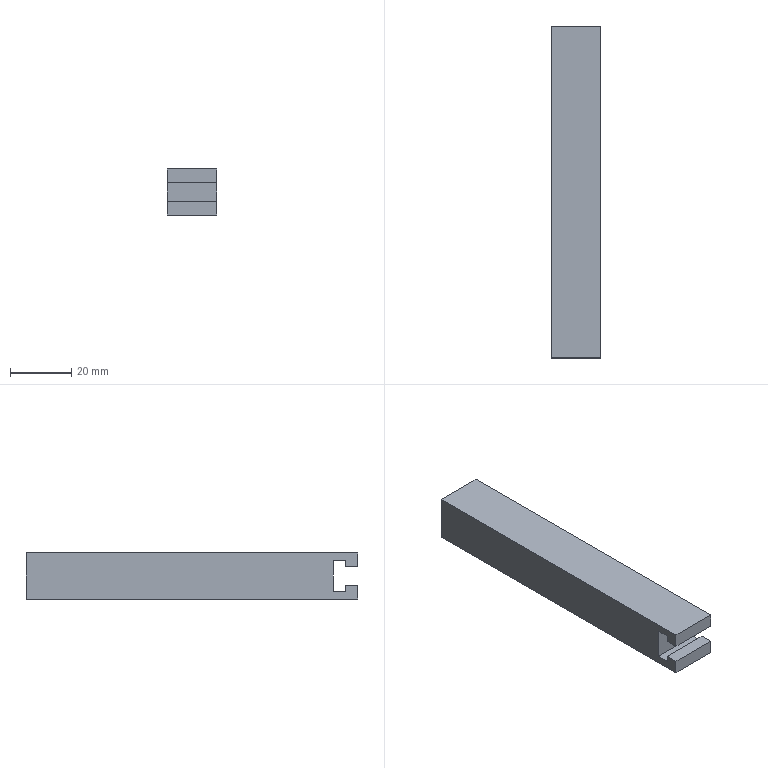Part | STEP file | 1 solid | 14 faces | box 16 x 108 x 15 mm | volume 24896 mm3 | plane 14
STEP:
#1=CARTESIAN_POINT('',(0.,0.,0.));
#2=DIRECTION('',(0.,0.,1.));
#3=DIRECTION('',(1.,0.,0.));
#4=AXIS2_PLACEMENT_3D('',#1,#2,#3);
#5=CARTESIAN_POINT('',(2.381,182.5,152.951));
#6=VERTEX_POINT('',#5);
#7=CARTESIAN_POINT('',(2.381,182.5,157.451));
#8=VERTEX_POINT('',#7);
#9=CARTESIAN_POINT('',(2.381,182.5,153.451));
#10=DIRECTION('',(0.,0.,1.));
#11=VECTOR('',#10,1.);
#12=LINE('',#9,#11);
#13=CARTESIAN_POINT('',(-5.619,182.5,153.451));
#14=DIRECTION('',(0.,-1.,0.));
#15=DIRECTION('',(0.,0.,-1.));
#16=AXIS2_PLACEMENT_3D('',#13,#14,#15);
#17=PLANE('',#16);
#18=CARTESIAN_POINT('',(0.,8.));
#19=DIRECTION('',(-1.,0.));
#20=VECTOR('',#19,1.);
#21=LINE('',#18,#20);
#22=(GEOMETRIC_REPRESENTATION_CONTEXT(2)PARAMETRIC_REPRESENTATION_CONTEXT()REPRESENTATION_CONTEXT('',''));
#23=DEFINITIONAL_REPRESENTATION('',(#21),#22);
#24=PCURVE('',#17,#23);
#25=CARTESIAN_POINT('',(2.381,130.5,152.951));
#26=DIRECTION('',(1.,0.,0.));
#27=DIRECTION('',(0.,0.,-1.));
#28=AXIS2_PLACEMENT_3D('',#25,#26,#27);
#29=PLANE('',#28);
#30=CARTESIAN_POINT('',(-0.5,52.));
#31=DIRECTION('',(-1.,0.));
#32=VECTOR('',#31,1.);
#33=LINE('',#30,#32);
#34=(GEOMETRIC_REPRESENTATION_CONTEXT(2)PARAMETRIC_REPRESENTATION_CONTEXT()REPRESENTATION_CONTEXT('',''));
#35=DEFINITIONAL_REPRESENTATION('',(#33),#34);
#36=PCURVE('',#29,#35);
#37=SURFACE_CURVE('',#12,(#24,#36),.PCURVE_S1.);
#38=EDGE_CURVE('',#6,#8,#37,.T.);
#39=ORIENTED_EDGE('',*,*,#38,.T.);
#40=CARTESIAN_POINT('',(-13.619,182.5,157.451));
#41=VERTEX_POINT('',#40);
#42=CARTESIAN_POINT('',(37.138,182.5,157.451));
#43=DIRECTION('',(-1.,0.,0.));
#44=VECTOR('',#43,1.);
#45=LINE('',#42,#44);
#46=CARTESIAN_POINT('',(-4.,42.756));
#47=DIRECTION('',(0.,-1.));
#48=VECTOR('',#47,1.);
#49=LINE('',#46,#48);
#50=(GEOMETRIC_REPRESENTATION_CONTEXT(2)PARAMETRIC_REPRESENTATION_CONTEXT()REPRESENTATION_CONTEXT('',''));
#51=DEFINITIONAL_REPRESENTATION('',(#49),#50);
#52=PCURVE('',#17,#51);
#53=CARTESIAN_POINT('',(37.138,95.5,157.451));
#54=DIRECTION('',(0.,0.,1.));
#55=DIRECTION('',(-1.,0.,0.));
#56=AXIS2_PLACEMENT_3D('',#53,#54,#55);
#57=PLANE('',#56);
#58=CARTESIAN_POINT('',(0.,-87.));
#59=DIRECTION('',(1.,0.));
#60=VECTOR('',#59,1.);
#61=LINE('',#58,#60);
#62=(GEOMETRIC_REPRESENTATION_CONTEXT(2)PARAMETRIC_REPRESENTATION_CONTEXT()REPRESENTATION_CONTEXT('',''));
#63=DEFINITIONAL_REPRESENTATION('',(#61),#62);
#64=PCURVE('',#57,#63);
#65=SURFACE_CURVE('',#45,(#52,#64),.PCURVE_S1.);
#66=EDGE_CURVE('',#8,#41,#65,.T.);
#67=ORIENTED_EDGE('',*,*,#66,.T.);
#68=CARTESIAN_POINT('',(-13.619,182.5,152.951));
#69=VERTEX_POINT('',#68);
#70=CARTESIAN_POINT('',(-13.619,182.5,153.451));
#71=DIRECTION('',(0.,0.,1.));
#72=VECTOR('',#71,1.);
#73=LINE('',#70,#72);
#74=CARTESIAN_POINT('',(0.,-8.));
#75=DIRECTION('',(-1.,0.));
#76=VECTOR('',#75,1.);
#77=LINE('',#74,#76);
#78=(GEOMETRIC_REPRESENTATION_CONTEXT(2)PARAMETRIC_REPRESENTATION_CONTEXT()REPRESENTATION_CONTEXT('',''));
#79=DEFINITIONAL_REPRESENTATION('',(#77),#78);
#80=PCURVE('',#17,#79);
#81=CARTESIAN_POINT('',(-13.619,130.5,152.951));
#82=DIRECTION('',(1.,0.,0.));
#83=DIRECTION('',(0.,0.,-1.));
#84=AXIS2_PLACEMENT_3D('',#81,#82,#83);
#85=PLANE('',#84);
#86=CARTESIAN_POINT('',(-0.5,52.));
#87=DIRECTION('',(-1.,0.));
#88=VECTOR('',#87,1.);
#89=LINE('',#86,#88);
#90=(GEOMETRIC_REPRESENTATION_CONTEXT(2)PARAMETRIC_REPRESENTATION_CONTEXT()REPRESENTATION_CONTEXT('',''));
#91=DEFINITIONAL_REPRESENTATION('',(#89),#90);
#92=PCURVE('',#85,#91);
#93=SURFACE_CURVE('',#73,(#80,#92),.PCURVE_S1.);
#94=EDGE_CURVE('',#69,#41,#93,.T.);
#95=ORIENTED_EDGE('',*,*,#94,.F.);
#96=CARTESIAN_POINT('',(-5.619,182.5,152.951));
#97=DIRECTION('',(1.,0.,0.));
#98=VECTOR('',#97,1.);
#99=LINE('',#96,#98);
#100=CARTESIAN_POINT('',(0.5,0.));
#101=DIRECTION('',(0.,1.));
#102=VECTOR('',#101,1.);
#103=LINE('',#100,#102);
#104=(GEOMETRIC_REPRESENTATION_CONTEXT(2)PARAMETRIC_REPRESENTATION_CONTEXT()REPRESENTATION_CONTEXT('',''));
#105=DEFINITIONAL_REPRESENTATION('',(#103),#104);
#106=PCURVE('',#17,#105);
#107=CARTESIAN_POINT('',(-5.619,165.5,152.951));
#108=DIRECTION('',(0.,0.,-1.));
#109=DIRECTION('',(-1.,0.,0.));
#110=AXIS2_PLACEMENT_3D('',#107,#108,#109);
#111=PLANE('',#110);
#112=CARTESIAN_POINT('',(0.,17.));
#113=DIRECTION('',(-1.,0.));
#114=VECTOR('',#113,1.);
#115=LINE('',#112,#114);
#116=(GEOMETRIC_REPRESENTATION_CONTEXT(2)PARAMETRIC_REPRESENTATION_CONTEXT()REPRESENTATION_CONTEXT('',''));
#117=DEFINITIONAL_REPRESENTATION('',(#115),#116);
#118=PCURVE('',#111,#117);
#119=SURFACE_CURVE('',#99,(#106,#118),.PCURVE_S1.);
#120=EDGE_CURVE('',#69,#6,#119,.T.);
#121=ORIENTED_EDGE('',*,*,#120,.T.);
#122=EDGE_LOOP('',(#39,#67,#95,#121));
#123=FACE_BOUND('',#122,.T.);
#124=ADVANCED_FACE('',(#123),#17,.T.);
#125=CARTESIAN_POINT('',(2.381,186.5,155.451));
#126=VERTEX_POINT('',#125);
#127=CARTESIAN_POINT('',(2.381,186.5,157.451));
#128=VERTEX_POINT('',#127);
#129=CARTESIAN_POINT('',(2.381,186.5,152.951));
#130=DIRECTION('',(0.,0.,1.));
#131=VECTOR('',#130,1.);
#132=LINE('',#129,#131);
#133=CARTESIAN_POINT('',(0.,56.));
#134=DIRECTION('',(-1.,0.));
#135=VECTOR('',#134,1.);
#136=LINE('',#133,#135);
#137=(GEOMETRIC_REPRESENTATION_CONTEXT(2)PARAMETRIC_REPRESENTATION_CONTEXT()REPRESENTATION_CONTEXT('',''));
#138=DEFINITIONAL_REPRESENTATION('',(#136),#137);
#139=PCURVE('',#29,#138);
#140=CARTESIAN_POINT('',(-142.714,186.5,160.451));
#141=DIRECTION('',(0.,1.,0.));
#142=DIRECTION('',(0.,0.,1.));
#143=AXIS2_PLACEMENT_3D('',#140,#141,#142);
#144=PLANE('',#143);
#145=CARTESIAN_POINT('',(-7.5,145.095));
#146=DIRECTION('',(1.,0.));
#147=VECTOR('',#146,1.);
#148=LINE('',#145,#147);
#149=(GEOMETRIC_REPRESENTATION_CONTEXT(2)PARAMETRIC_REPRESENTATION_CONTEXT()REPRESENTATION_CONTEXT('',''));
#150=DEFINITIONAL_REPRESENTATION('',(#148),#149);
#151=PCURVE('',#144,#150);
#152=SURFACE_CURVE('',#132,(#139,#151),.PCURVE_S1.);
#153=EDGE_CURVE('',#126,#128,#152,.T.);
#154=ORIENTED_EDGE('',*,*,#153,.T.);
#155=CARTESIAN_POINT('',(2.381,130.5,157.451));
#156=DIRECTION('',(0.,-1.,0.));
#157=VECTOR('',#156,1.);
#158=LINE('',#155,#157);
#159=CARTESIAN_POINT('',(-4.5,0.));
#160=DIRECTION('',(0.,-1.));
#161=VECTOR('',#160,1.);
#162=LINE('',#159,#161);
#163=(GEOMETRIC_REPRESENTATION_CONTEXT(2)PARAMETRIC_REPRESENTATION_CONTEXT()REPRESENTATION_CONTEXT('',''));
#164=DEFINITIONAL_REPRESENTATION('',(#162),#163);
#165=PCURVE('',#29,#164);
#166=CARTESIAN_POINT('',(34.756,-35.));
#167=DIRECTION('',(0.,1.));
#168=VECTOR('',#167,1.);
#169=LINE('',#166,#168);
#170=(GEOMETRIC_REPRESENTATION_CONTEXT(2)PARAMETRIC_REPRESENTATION_CONTEXT()REPRESENTATION_CONTEXT('',''));
#171=DEFINITIONAL_REPRESENTATION('',(#169),#170);
#172=PCURVE('',#57,#171);
#173=SURFACE_CURVE('',#158,(#165,#172),.PCURVE_S1.);
#174=EDGE_CURVE('',#128,#8,#173,.T.);
#175=ORIENTED_EDGE('',*,*,#174,.T.);
#176=ORIENTED_EDGE('',*,*,#38,.F.);
#177=CARTESIAN_POINT('',(2.381,290.5,152.951));
#178=VERTEX_POINT('',#177);
#179=CARTESIAN_POINT('',(2.381,165.5,152.951));
#180=DIRECTION('',(0.,-1.,0.));
#181=VECTOR('',#180,1.);
#182=LINE('',#179,#181);
#183=CARTESIAN_POINT('',(0.,35.));
#184=DIRECTION('',(0.,-1.));
#185=VECTOR('',#184,1.);
#186=LINE('',#183,#185);
#187=(GEOMETRIC_REPRESENTATION_CONTEXT(2)PARAMETRIC_REPRESENTATION_CONTEXT()REPRESENTATION_CONTEXT('',''));
#188=DEFINITIONAL_REPRESENTATION('',(#186),#187);
#189=PCURVE('',#29,#188);
#190=CARTESIAN_POINT('',(-8.,0.));
#191=DIRECTION('',(0.,-1.));
#192=VECTOR('',#191,1.);
#193=LINE('',#190,#192);
#194=(GEOMETRIC_REPRESENTATION_CONTEXT(2)PARAMETRIC_REPRESENTATION_CONTEXT()REPRESENTATION_CONTEXT('',''));
#195=DEFINITIONAL_REPRESENTATION('',(#193),#194);
#196=PCURVE('',#111,#195);
#197=SURFACE_CURVE('',#182,(#189,#196),.PCURVE_S1.);
#198=EDGE_CURVE('',#178,#6,#197,.T.);
#199=ORIENTED_EDGE('',*,*,#198,.F.);
#200=CARTESIAN_POINT('',(2.381,290.5,167.951));
#201=VERTEX_POINT('',#200);
#202=CARTESIAN_POINT('',(2.381,290.5,153.451));
#203=DIRECTION('',(0.,0.,-1.));
#204=VECTOR('',#203,1.);
#205=LINE('',#202,#204);
#206=CARTESIAN_POINT('',(-0.5,160.));
#207=DIRECTION('',(1.,0.));
#208=VECTOR('',#207,1.);
#209=LINE('',#206,#208);
#210=(GEOMETRIC_REPRESENTATION_CONTEXT(2)PARAMETRIC_REPRESENTATION_CONTEXT()REPRESENTATION_CONTEXT('',''));
#211=DEFINITIONAL_REPRESENTATION('',(#209),#210);
#212=PCURVE('',#29,#211);
#213=CARTESIAN_POINT('',(-5.619,290.5,153.451));
#214=DIRECTION('',(0.,1.,0.));
#215=DIRECTION('',(0.,0.,1.));
#216=AXIS2_PLACEMENT_3D('',#213,#214,#215);
#217=PLANE('',#216);
#218=CARTESIAN_POINT('',(0.,8.));
#219=DIRECTION('',(-1.,0.));
#220=VECTOR('',#219,1.);
#221=LINE('',#218,#220);
#222=(GEOMETRIC_REPRESENTATION_CONTEXT(2)PARAMETRIC_REPRESENTATION_CONTEXT()REPRESENTATION_CONTEXT('',''));
#223=DEFINITIONAL_REPRESENTATION('',(#221),#222);
#224=PCURVE('',#217,#223);
#225=SURFACE_CURVE('',#205,(#212,#224),.PCURVE_S1.);
#226=EDGE_CURVE('',#201,#178,#225,.T.);
#227=ORIENTED_EDGE('',*,*,#226,.F.);
#228=CARTESIAN_POINT('',(2.381,182.5,167.951));
#229=VERTEX_POINT('',#228);
#230=CARTESIAN_POINT('',(2.381,165.5,167.951));
#231=DIRECTION('',(0.,1.,0.));
#232=VECTOR('',#231,1.);
#233=LINE('',#230,#232);
#234=CARTESIAN_POINT('',(-15.,35.));
#235=DIRECTION('',(0.,1.));
#236=VECTOR('',#235,1.);
#237=LINE('',#234,#236);
#238=(GEOMETRIC_REPRESENTATION_CONTEXT(2)PARAMETRIC_REPRESENTATION_CONTEXT()REPRESENTATION_CONTEXT('',''));
#239=DEFINITIONAL_REPRESENTATION('',(#237),#238);
#240=PCURVE('',#29,#239);
#241=CARTESIAN_POINT('',(-5.619,165.5,167.951));
#242=DIRECTION('',(0.,0.,1.));
#243=DIRECTION('',(1.,0.,0.));
#244=AXIS2_PLACEMENT_3D('',#241,#242,#243);
#245=PLANE('',#244);
#246=CARTESIAN_POINT('',(8.,0.));
#247=DIRECTION('',(0.,1.));
#248=VECTOR('',#247,1.);
#249=LINE('',#246,#248);
#250=(GEOMETRIC_REPRESENTATION_CONTEXT(2)PARAMETRIC_REPRESENTATION_CONTEXT()REPRESENTATION_CONTEXT('',''));
#251=DEFINITIONAL_REPRESENTATION('',(#249),#250);
#252=PCURVE('',#245,#251);
#253=SURFACE_CURVE('',#233,(#240,#252),.PCURVE_S1.);
#254=EDGE_CURVE('',#229,#201,#253,.T.);
#255=ORIENTED_EDGE('',*,*,#254,.F.);
#256=CARTESIAN_POINT('',(2.381,182.5,163.451));
#257=VERTEX_POINT('',#256);
#258=CARTESIAN_POINT('',(2.381,182.5,153.451));
#259=DIRECTION('',(0.,0.,1.));
#260=VECTOR('',#259,1.);
#261=LINE('',#258,#260);
#262=CARTESIAN_POINT('',(-0.5,52.));
#263=DIRECTION('',(-1.,0.));
#264=VECTOR('',#263,1.);
#265=LINE('',#262,#264);
#266=(GEOMETRIC_REPRESENTATION_CONTEXT(2)PARAMETRIC_REPRESENTATION_CONTEXT()REPRESENTATION_CONTEXT('',''));
#267=DEFINITIONAL_REPRESENTATION('',(#265),#266);
#268=PCURVE('',#29,#267);
#269=CARTESIAN_POINT('',(-5.619,182.5,153.451));
#270=DIRECTION('',(0.,-1.,0.));
#271=DIRECTION('',(0.,0.,-1.));
#272=AXIS2_PLACEMENT_3D('',#269,#270,#271);
#273=PLANE('',#272);
#274=CARTESIAN_POINT('',(0.,8.));
#275=DIRECTION('',(-1.,0.));
#276=VECTOR('',#275,1.);
#277=LINE('',#274,#276);
#278=(GEOMETRIC_REPRESENTATION_CONTEXT(2)PARAMETRIC_REPRESENTATION_CONTEXT()REPRESENTATION_CONTEXT('',''));
#279=DEFINITIONAL_REPRESENTATION('',(#277),#278);
#280=PCURVE('',#273,#279);
#281=SURFACE_CURVE('',#261,(#268,#280),.PCURVE_S1.);
#282=EDGE_CURVE('',#257,#229,#281,.T.);
#283=ORIENTED_EDGE('',*,*,#282,.F.);
#284=CARTESIAN_POINT('',(2.381,186.5,163.451));
#285=VERTEX_POINT('',#284);
#286=CARTESIAN_POINT('',(2.381,130.5,163.451));
#287=DIRECTION('',(0.,-1.,0.));
#288=VECTOR('',#287,1.);
#289=LINE('',#286,#288);
#290=CARTESIAN_POINT('',(-10.5,0.));
#291=DIRECTION('',(0.,-1.));
#292=VECTOR('',#291,1.);
#293=LINE('',#290,#292);
#294=(GEOMETRIC_REPRESENTATION_CONTEXT(2)PARAMETRIC_REPRESENTATION_CONTEXT()REPRESENTATION_CONTEXT('',''));
#295=DEFINITIONAL_REPRESENTATION('',(#293),#294);
#296=PCURVE('',#29,#295);
#297=CARTESIAN_POINT('',(37.138,95.5,163.451));
#298=DIRECTION('',(0.,0.,1.));
#299=DIRECTION('',(-1.,0.,0.));
#300=AXIS2_PLACEMENT_3D('',#297,#298,#299);
#301=PLANE('',#300);
#302=CARTESIAN_POINT('',(34.756,-35.));
#303=DIRECTION('',(0.,1.));
#304=VECTOR('',#303,1.);
#305=LINE('',#302,#304);
#306=(GEOMETRIC_REPRESENTATION_CONTEXT(2)PARAMETRIC_REPRESENTATION_CONTEXT()REPRESENTATION_CONTEXT('',''));
#307=DEFINITIONAL_REPRESENTATION('',(#305),#306);
#308=PCURVE('',#301,#307);
#309=SURFACE_CURVE('',#289,(#296,#308),.PCURVE_S1.);
#310=EDGE_CURVE('',#285,#257,#309,.T.);
#311=ORIENTED_EDGE('',*,*,#310,.F.);
#312=CARTESIAN_POINT('',(2.381,186.5,165.451));
#313=VERTEX_POINT('',#312);
#314=CARTESIAN_POINT('',(2.381,186.5,152.951));
#315=DIRECTION('',(0.,0.,1.));
#316=VECTOR('',#315,1.);
#317=LINE('',#314,#316);
#318=CARTESIAN_POINT('',(0.,56.));
#319=DIRECTION('',(-1.,0.));
#320=VECTOR('',#319,1.);
#321=LINE('',#318,#320);
#322=(GEOMETRIC_REPRESENTATION_CONTEXT(2)PARAMETRIC_REPRESENTATION_CONTEXT()REPRESENTATION_CONTEXT('',''));
#323=DEFINITIONAL_REPRESENTATION('',(#321),#322);
#324=PCURVE('',#29,#323);
#325=CARTESIAN_POINT('',(-142.714,186.5,160.451));
#326=DIRECTION('',(0.,1.,0.));
#327=DIRECTION('',(0.,0.,1.));
#328=AXIS2_PLACEMENT_3D('',#325,#326,#327);
#329=PLANE('',#328);
#330=CARTESIAN_POINT('',(-7.5,145.095));
#331=DIRECTION('',(1.,0.));
#332=VECTOR('',#331,1.);
#333=LINE('',#330,#332);
#334=(GEOMETRIC_REPRESENTATION_CONTEXT(2)PARAMETRIC_REPRESENTATION_CONTEXT()REPRESENTATION_CONTEXT('',''));
#335=DEFINITIONAL_REPRESENTATION('',(#333),#334);
#336=PCURVE('',#329,#335);
#337=SURFACE_CURVE('',#317,(#324,#336),.PCURVE_S1.);
#338=EDGE_CURVE('',#285,#313,#337,.T.);
#339=ORIENTED_EDGE('',*,*,#338,.T.);
#340=CARTESIAN_POINT('',(2.381,190.5,165.451));
#341=VERTEX_POINT('',#340);
#342=CARTESIAN_POINT('',(2.381,130.5,165.451));
#343=DIRECTION('',(0.,-1.,0.));
#344=VECTOR('',#343,1.);
#345=LINE('',#342,#344);
#346=CARTESIAN_POINT('',(-12.5,0.));
#347=DIRECTION('',(0.,-1.));
#348=VECTOR('',#347,1.);
#349=LINE('',#346,#348);
#350=(GEOMETRIC_REPRESENTATION_CONTEXT(2)PARAMETRIC_REPRESENTATION_CONTEXT()REPRESENTATION_CONTEXT('',''));
#351=DEFINITIONAL_REPRESENTATION('',(#349),#350);
#352=PCURVE('',#29,#351);
#353=CARTESIAN_POINT('',(37.138,95.5,165.451));
#354=DIRECTION('',(0.,0.,1.));
#355=DIRECTION('',(-1.,0.,0.));
#356=AXIS2_PLACEMENT_3D('',#353,#354,#355);
#357=PLANE('',#356);
#358=CARTESIAN_POINT('',(34.756,-35.));
#359=DIRECTION('',(0.,1.));
#360=VECTOR('',#359,1.);
#361=LINE('',#358,#360);
#362=(GEOMETRIC_REPRESENTATION_CONTEXT(2)PARAMETRIC_REPRESENTATION_CONTEXT()REPRESENTATION_CONTEXT('',''));
#363=DEFINITIONAL_REPRESENTATION('',(#361),#362);
#364=PCURVE('',#357,#363);
#365=SURFACE_CURVE('',#345,(#352,#364),.PCURVE_S1.);
#366=EDGE_CURVE('',#341,#313,#365,.T.);
#367=ORIENTED_EDGE('',*,*,#366,.F.);
#368=CARTESIAN_POINT('',(2.381,190.5,155.451));
#369=VERTEX_POINT('',#368);
#370=CARTESIAN_POINT('',(2.381,190.5,152.951));
#371=DIRECTION('',(0.,0.,1.));
#372=VECTOR('',#371,1.);
#373=LINE('',#370,#372);
#374=CARTESIAN_POINT('',(0.,60.));
#375=DIRECTION('',(-1.,0.));
#376=VECTOR('',#375,1.);
#377=LINE('',#374,#376);
#378=(GEOMETRIC_REPRESENTATION_CONTEXT(2)PARAMETRIC_REPRESENTATION_CONTEXT()REPRESENTATION_CONTEXT('',''));
#379=DEFINITIONAL_REPRESENTATION('',(#377),#378);
#380=PCURVE('',#29,#379);
#381=CARTESIAN_POINT('',(-72.862,190.5,108.53));
#382=DIRECTION('',(0.,1.,0.));
#383=DIRECTION('',(0.,0.,1.));
#384=AXIS2_PLACEMENT_3D('',#381,#382,#383);
#385=PLANE('',#384);
#386=CARTESIAN_POINT('',(44.422,75.244));
#387=DIRECTION('',(1.,0.));
#388=VECTOR('',#387,1.);
#389=LINE('',#386,#388);
#390=(GEOMETRIC_REPRESENTATION_CONTEXT(2)PARAMETRIC_REPRESENTATION_CONTEXT()REPRESENTATION_CONTEXT('',''));
#391=DEFINITIONAL_REPRESENTATION('',(#389),#390);
#392=PCURVE('',#385,#391);
#393=SURFACE_CURVE('',#373,(#380,#392),.PCURVE_S1.);
#394=EDGE_CURVE('',#369,#341,#393,.T.);
#395=ORIENTED_EDGE('',*,*,#394,.F.);
#396=CARTESIAN_POINT('',(2.381,130.5,155.451));
#397=DIRECTION('',(0.,-1.,0.));
#398=VECTOR('',#397,1.);
#399=LINE('',#396,#398);
#400=CARTESIAN_POINT('',(-2.5,0.));
#401=DIRECTION('',(0.,-1.));
#402=VECTOR('',#401,1.);
#403=LINE('',#400,#402);
#404=(GEOMETRIC_REPRESENTATION_CONTEXT(2)PARAMETRIC_REPRESENTATION_CONTEXT()REPRESENTATION_CONTEXT('',''));
#405=DEFINITIONAL_REPRESENTATION('',(#403),#404);
#406=PCURVE('',#29,#405);
#407=CARTESIAN_POINT('',(37.138,95.5,155.451));
#408=DIRECTION('',(0.,0.,1.));
#409=DIRECTION('',(-1.,0.,0.));
#410=AXIS2_PLACEMENT_3D('',#407,#408,#409);
#411=PLANE('',#410);
#412=CARTESIAN_POINT('',(34.756,-35.));
#413=DIRECTION('',(0.,1.));
#414=VECTOR('',#413,1.);
#415=LINE('',#412,#414);
#416=(GEOMETRIC_REPRESENTATION_CONTEXT(2)PARAMETRIC_REPRESENTATION_CONTEXT()REPRESENTATION_CONTEXT('',''));
#417=DEFINITIONAL_REPRESENTATION('',(#415),#416);
#418=PCURVE('',#411,#417);
#419=SURFACE_CURVE('',#399,(#406,#418),.PCURVE_S1.);
#420=EDGE_CURVE('',#369,#126,#419,.T.);
#421=ORIENTED_EDGE('',*,*,#420,.T.);
#422=EDGE_LOOP('',(#154,#175,#176,#199,#227,#255,#283,#311,#339,#367,#395,#421));
#423=FACE_BOUND('',#422,.T.);
#424=ADVANCED_FACE('',(#423),#29,.T.);
#425=CARTESIAN_POINT('',(-13.619,186.5,157.451));
#426=VERTEX_POINT('',#425);
#427=CARTESIAN_POINT('',(-13.619,130.5,157.451));
#428=DIRECTION('',(0.,-1.,0.));
#429=VECTOR('',#428,1.);
#430=LINE('',#427,#429);
#431=CARTESIAN_POINT('',(-4.5,0.));
#432=DIRECTION('',(0.,-1.));
#433=VECTOR('',#432,1.);
#434=LINE('',#431,#433);
#435=(GEOMETRIC_REPRESENTATION_CONTEXT(2)PARAMETRIC_REPRESENTATION_CONTEXT()REPRESENTATION_CONTEXT('',''));
#436=DEFINITIONAL_REPRESENTATION('',(#434),#435);
#437=PCURVE('',#85,#436);
#438=CARTESIAN_POINT('',(50.756,-35.));
#439=DIRECTION('',(0.,1.));
#440=VECTOR('',#439,1.);
#441=LINE('',#438,#440);
#442=(GEOMETRIC_REPRESENTATION_CONTEXT(2)PARAMETRIC_REPRESENTATION_CONTEXT()REPRESENTATION_CONTEXT('',''));
#443=DEFINITIONAL_REPRESENTATION('',(#441),#442);
#444=PCURVE('',#57,#443);
#445=SURFACE_CURVE('',#430,(#437,#444),.PCURVE_S1.);
#446=EDGE_CURVE('',#426,#41,#445,.T.);
#447=ORIENTED_EDGE('',*,*,#446,.F.);
#448=CARTESIAN_POINT('',(-13.619,186.5,155.451));
#449=VERTEX_POINT('',#448);
#450=CARTESIAN_POINT('',(-13.619,186.5,152.951));
#451=DIRECTION('',(0.,0.,1.));
#452=VECTOR('',#451,1.);
#453=LINE('',#450,#452);
#454=CARTESIAN_POINT('',(0.,56.));
#455=DIRECTION('',(-1.,0.));
#456=VECTOR('',#455,1.);
#457=LINE('',#454,#456);
#458=(GEOMETRIC_REPRESENTATION_CONTEXT(2)PARAMETRIC_REPRESENTATION_CONTEXT()REPRESENTATION_CONTEXT('',''));
#459=DEFINITIONAL_REPRESENTATION('',(#457),#458);
#460=PCURVE('',#85,#459);
#461=CARTESIAN_POINT('',(-7.5,129.095));
#462=DIRECTION('',(1.,0.));
#463=VECTOR('',#462,1.);
#464=LINE('',#461,#463);
#465=(GEOMETRIC_REPRESENTATION_CONTEXT(2)PARAMETRIC_REPRESENTATION_CONTEXT()REPRESENTATION_CONTEXT('',''));
#466=DEFINITIONAL_REPRESENTATION('',(#464),#465);
#467=PCURVE('',#144,#466);
#468=SURFACE_CURVE('',#453,(#460,#467),.PCURVE_S1.);
#469=EDGE_CURVE('',#449,#426,#468,.T.);
#470=ORIENTED_EDGE('',*,*,#469,.F.);
#471=CARTESIAN_POINT('',(-13.619,190.5,155.451));
#472=VERTEX_POINT('',#471);
#473=CARTESIAN_POINT('',(-13.619,130.5,155.451));
#474=DIRECTION('',(0.,-1.,0.));
#475=VECTOR('',#474,1.);
#476=LINE('',#473,#475);
#477=CARTESIAN_POINT('',(-2.5,0.));
#478=DIRECTION('',(0.,-1.));
#479=VECTOR('',#478,1.);
#480=LINE('',#477,#479);
#481=(GEOMETRIC_REPRESENTATION_CONTEXT(2)PARAMETRIC_REPRESENTATION_CONTEXT()REPRESENTATION_CONTEXT('',''));
#482=DEFINITIONAL_REPRESENTATION('',(#480),#481);
#483=PCURVE('',#85,#482);
#484=CARTESIAN_POINT('',(50.756,-35.));
#485=DIRECTION('',(0.,1.));
#486=VECTOR('',#485,1.);
#487=LINE('',#484,#486);
#488=(GEOMETRIC_REPRESENTATION_CONTEXT(2)PARAMETRIC_REPRESENTATION_CONTEXT()REPRESENTATION_CONTEXT('',''));
#489=DEFINITIONAL_REPRESENTATION('',(#487),#488);
#490=PCURVE('',#411,#489);
#491=SURFACE_CURVE('',#476,(#483,#490),.PCURVE_S1.);
#492=EDGE_CURVE('',#472,#449,#491,.T.);
#493=ORIENTED_EDGE('',*,*,#492,.F.);
#494=CARTESIAN_POINT('',(-13.619,190.5,165.451));
#495=VERTEX_POINT('',#494);
#496=CARTESIAN_POINT('',(-13.619,190.5,152.951));
#497=DIRECTION('',(0.,0.,1.));
#498=VECTOR('',#497,1.);
#499=LINE('',#496,#498);
#500=CARTESIAN_POINT('',(0.,60.));
#501=DIRECTION('',(-1.,0.));
#502=VECTOR('',#501,1.);
#503=LINE('',#500,#502);
#504=(GEOMETRIC_REPRESENTATION_CONTEXT(2)PARAMETRIC_REPRESENTATION_CONTEXT()REPRESENTATION_CONTEXT('',''));
#505=DEFINITIONAL_REPRESENTATION('',(#503),#504);
#506=PCURVE('',#85,#505);
#507=CARTESIAN_POINT('',(44.422,59.244));
#508=DIRECTION('',(1.,0.));
#509=VECTOR('',#508,1.);
#510=LINE('',#507,#509);
#511=(GEOMETRIC_REPRESENTATION_CONTEXT(2)PARAMETRIC_REPRESENTATION_CONTEXT()REPRESENTATION_CONTEXT('',''));
#512=DEFINITIONAL_REPRESENTATION('',(#510),#511);
#513=PCURVE('',#385,#512);
#514=SURFACE_CURVE('',#499,(#506,#513),.PCURVE_S1.);
#515=EDGE_CURVE('',#472,#495,#514,.T.);
#516=ORIENTED_EDGE('',*,*,#515,.T.);
#517=CARTESIAN_POINT('',(-13.619,186.5,165.451));
#518=VERTEX_POINT('',#517);
#519=CARTESIAN_POINT('',(-13.619,130.5,165.451));
#520=DIRECTION('',(0.,-1.,0.));
#521=VECTOR('',#520,1.);
#522=LINE('',#519,#521);
#523=CARTESIAN_POINT('',(-12.5,0.));
#524=DIRECTION('',(0.,-1.));
#525=VECTOR('',#524,1.);
#526=LINE('',#523,#525);
#527=(GEOMETRIC_REPRESENTATION_CONTEXT(2)PARAMETRIC_REPRESENTATION_CONTEXT()REPRESENTATION_CONTEXT('',''));
#528=DEFINITIONAL_REPRESENTATION('',(#526),#527);
#529=PCURVE('',#85,#528);
#530=CARTESIAN_POINT('',(50.756,-35.));
#531=DIRECTION('',(0.,1.));
#532=VECTOR('',#531,1.);
#533=LINE('',#530,#532);
#534=(GEOMETRIC_REPRESENTATION_CONTEXT(2)PARAMETRIC_REPRESENTATION_CONTEXT()REPRESENTATION_CONTEXT('',''));
#535=DEFINITIONAL_REPRESENTATION('',(#533),#534);
#536=PCURVE('',#357,#535);
#537=SURFACE_CURVE('',#522,(#529,#536),.PCURVE_S1.);
#538=EDGE_CURVE('',#495,#518,#537,.T.);
#539=ORIENTED_EDGE('',*,*,#538,.T.);
#540=CARTESIAN_POINT('',(-13.619,186.5,163.451));
#541=VERTEX_POINT('',#540);
#542=CARTESIAN_POINT('',(-13.619,186.5,152.951));
#543=DIRECTION('',(0.,0.,1.));
#544=VECTOR('',#543,1.);
#545=LINE('',#542,#544);
#546=CARTESIAN_POINT('',(0.,56.));
#547=DIRECTION('',(-1.,0.));
#548=VECTOR('',#547,1.);
#549=LINE('',#546,#548);
#550=(GEOMETRIC_REPRESENTATION_CONTEXT(2)PARAMETRIC_REPRESENTATION_CONTEXT()REPRESENTATION_CONTEXT('',''));
#551=DEFINITIONAL_REPRESENTATION('',(#549),#550);
#552=PCURVE('',#85,#551);
#553=CARTESIAN_POINT('',(-7.5,129.095));
#554=DIRECTION('',(1.,0.));
#555=VECTOR('',#554,1.);
#556=LINE('',#553,#555);
#557=(GEOMETRIC_REPRESENTATION_CONTEXT(2)PARAMETRIC_REPRESENTATION_CONTEXT()REPRESENTATION_CONTEXT('',''));
#558=DEFINITIONAL_REPRESENTATION('',(#556),#557);
#559=PCURVE('',#329,#558);
#560=SURFACE_CURVE('',#545,(#552,#559),.PCURVE_S1.);
#561=EDGE_CURVE('',#541,#518,#560,.T.);
#562=ORIENTED_EDGE('',*,*,#561,.F.);
#563=CARTESIAN_POINT('',(-13.619,182.5,163.451));
#564=VERTEX_POINT('',#563);
#565=CARTESIAN_POINT('',(-13.619,130.5,163.451));
#566=DIRECTION('',(0.,-1.,0.));
#567=VECTOR('',#566,1.);
#568=LINE('',#565,#567);
#569=CARTESIAN_POINT('',(-10.5,0.));
#570=DIRECTION('',(0.,-1.));
#571=VECTOR('',#570,1.);
#572=LINE('',#569,#571);
#573=(GEOMETRIC_REPRESENTATION_CONTEXT(2)PARAMETRIC_REPRESENTATION_CONTEXT()REPRESENTATION_CONTEXT('',''));
#574=DEFINITIONAL_REPRESENTATION('',(#572),#573);
#575=PCURVE('',#85,#574);
#576=CARTESIAN_POINT('',(50.756,-35.));
#577=DIRECTION('',(0.,1.));
#578=VECTOR('',#577,1.);
#579=LINE('',#576,#578);
#580=(GEOMETRIC_REPRESENTATION_CONTEXT(2)PARAMETRIC_REPRESENTATION_CONTEXT()REPRESENTATION_CONTEXT('',''));
#581=DEFINITIONAL_REPRESENTATION('',(#579),#580);
#582=PCURVE('',#301,#581);
#583=SURFACE_CURVE('',#568,(#575,#582),.PCURVE_S1.);
#584=EDGE_CURVE('',#541,#564,#583,.T.);
#585=ORIENTED_EDGE('',*,*,#584,.T.);
#586=CARTESIAN_POINT('',(-13.619,182.5,167.951));
#587=VERTEX_POINT('',#586);
#588=CARTESIAN_POINT('',(-13.619,182.5,153.451));
#589=DIRECTION('',(0.,0.,1.));
#590=VECTOR('',#589,1.);
#591=LINE('',#588,#590);
#592=CARTESIAN_POINT('',(-0.5,52.));
#593=DIRECTION('',(-1.,0.));
#594=VECTOR('',#593,1.);
#595=LINE('',#592,#594);
#596=(GEOMETRIC_REPRESENTATION_CONTEXT(2)PARAMETRIC_REPRESENTATION_CONTEXT()REPRESENTATION_CONTEXT('',''));
#597=DEFINITIONAL_REPRESENTATION('',(#595),#596);
#598=PCURVE('',#85,#597);
#599=CARTESIAN_POINT('',(0.,-8.));
#600=DIRECTION('',(-1.,0.));
#601=VECTOR('',#600,1.);
#602=LINE('',#599,#601);
#603=(GEOMETRIC_REPRESENTATION_CONTEXT(2)PARAMETRIC_REPRESENTATION_CONTEXT()REPRESENTATION_CONTEXT('',''));
#604=DEFINITIONAL_REPRESENTATION('',(#602),#603);
#605=PCURVE('',#273,#604);
#606=SURFACE_CURVE('',#591,(#598,#605),.PCURVE_S1.);
#607=EDGE_CURVE('',#564,#587,#606,.T.);
#608=ORIENTED_EDGE('',*,*,#607,.T.);
#609=CARTESIAN_POINT('',(-13.619,290.5,167.951));
#610=VERTEX_POINT('',#609);
#611=CARTESIAN_POINT('',(-13.619,165.5,167.951));
#612=DIRECTION('',(0.,1.,0.));
#613=VECTOR('',#612,1.);
#614=LINE('',#611,#613);
#615=CARTESIAN_POINT('',(-15.,35.));
#616=DIRECTION('',(0.,1.));
#617=VECTOR('',#616,1.);
#618=LINE('',#615,#617);
#619=(GEOMETRIC_REPRESENTATION_CONTEXT(2)PARAMETRIC_REPRESENTATION_CONTEXT()REPRESENTATION_CONTEXT('',''));
#620=DEFINITIONAL_REPRESENTATION('',(#618),#619);
#621=PCURVE('',#85,#620);
#622=CARTESIAN_POINT('',(-8.,0.));
#623=DIRECTION('',(0.,1.));
#624=VECTOR('',#623,1.);
#625=LINE('',#622,#624);
#626=(GEOMETRIC_REPRESENTATION_CONTEXT(2)PARAMETRIC_REPRESENTATION_CONTEXT()REPRESENTATION_CONTEXT('',''));
#627=DEFINITIONAL_REPRESENTATION('',(#625),#626);
#628=PCURVE('',#245,#627);
#629=SURFACE_CURVE('',#614,(#621,#628),.PCURVE_S1.);
#630=EDGE_CURVE('',#587,#610,#629,.T.);
#631=ORIENTED_EDGE('',*,*,#630,.T.);
#632=CARTESIAN_POINT('',(-13.619,290.5,152.951));
#633=VERTEX_POINT('',#632);
#634=CARTESIAN_POINT('',(-13.619,290.5,153.451));
#635=DIRECTION('',(0.,0.,-1.));
#636=VECTOR('',#635,1.);
#637=LINE('',#634,#636);
#638=CARTESIAN_POINT('',(-0.5,160.));
#639=DIRECTION('',(1.,0.));
#640=VECTOR('',#639,1.);
#641=LINE('',#638,#640);
#642=(GEOMETRIC_REPRESENTATION_CONTEXT(2)PARAMETRIC_REPRESENTATION_CONTEXT()REPRESENTATION_CONTEXT('',''));
#643=DEFINITIONAL_REPRESENTATION('',(#641),#642);
#644=PCURVE('',#85,#643);
#645=CARTESIAN_POINT('',(0.,-8.));
#646=DIRECTION('',(-1.,0.));
#647=VECTOR('',#646,1.);
#648=LINE('',#645,#647);
#649=(GEOMETRIC_REPRESENTATION_CONTEXT(2)PARAMETRIC_REPRESENTATION_CONTEXT()REPRESENTATION_CONTEXT('',''));
#650=DEFINITIONAL_REPRESENTATION('',(#648),#649);
#651=PCURVE('',#217,#650);
#652=SURFACE_CURVE('',#637,(#644,#651),.PCURVE_S1.);
#653=EDGE_CURVE('',#610,#633,#652,.T.);
#654=ORIENTED_EDGE('',*,*,#653,.T.);
#655=CARTESIAN_POINT('',(-13.619,165.5,152.951));
#656=DIRECTION('',(0.,-1.,0.));
#657=VECTOR('',#656,1.);
#658=LINE('',#655,#657);
#659=CARTESIAN_POINT('',(0.,35.));
#660=DIRECTION('',(0.,-1.));
#661=VECTOR('',#660,1.);
#662=LINE('',#659,#661);
#663=(GEOMETRIC_REPRESENTATION_CONTEXT(2)PARAMETRIC_REPRESENTATION_CONTEXT()REPRESENTATION_CONTEXT('',''));
#664=DEFINITIONAL_REPRESENTATION('',(#662),#663);
#665=PCURVE('',#85,#664);
#666=CARTESIAN_POINT('',(8.,0.));
#667=DIRECTION('',(0.,-1.));
#668=VECTOR('',#667,1.);
#669=LINE('',#666,#668);
#670=(GEOMETRIC_REPRESENTATION_CONTEXT(2)PARAMETRIC_REPRESENTATION_CONTEXT()REPRESENTATION_CONTEXT('',''));
#671=DEFINITIONAL_REPRESENTATION('',(#669),#670);
#672=PCURVE('',#111,#671);
#673=SURFACE_CURVE('',#658,(#665,#672),.PCURVE_S1.);
#674=EDGE_CURVE('',#633,#69,#673,.T.);
#675=ORIENTED_EDGE('',*,*,#674,.T.);
#676=ORIENTED_EDGE('',*,*,#94,.T.);
#677=EDGE_LOOP('',(#447,#470,#493,#516,#539,#562,#585,#608,#631,#654,#675,#676));
#678=FACE_BOUND('',#677,.T.);
#679=ADVANCED_FACE('',(#678),#85,.F.);
#680=ORIENTED_EDGE('',*,*,#674,.F.);
#681=CARTESIAN_POINT('',(-5.619,290.5,152.951));
#682=DIRECTION('',(-1.,0.,0.));
#683=VECTOR('',#682,1.);
#684=LINE('',#681,#683);
#685=CARTESIAN_POINT('',(0.,125.));
#686=DIRECTION('',(1.,0.));
#687=VECTOR('',#686,1.);
#688=LINE('',#685,#687);
#689=(GEOMETRIC_REPRESENTATION_CONTEXT(2)PARAMETRIC_REPRESENTATION_CONTEXT()REPRESENTATION_CONTEXT('',''));
#690=DEFINITIONAL_REPRESENTATION('',(#688),#689);
#691=PCURVE('',#111,#690);
#692=CARTESIAN_POINT('',(-0.5,0.));
#693=DIRECTION('',(0.,-1.));
#694=VECTOR('',#693,1.);
#695=LINE('',#692,#694);
#696=(GEOMETRIC_REPRESENTATION_CONTEXT(2)PARAMETRIC_REPRESENTATION_CONTEXT()REPRESENTATION_CONTEXT('',''));
#697=DEFINITIONAL_REPRESENTATION('',(#695),#696);
#698=PCURVE('',#217,#697);
#699=SURFACE_CURVE('',#684,(#691,#698),.PCURVE_S1.);
#700=EDGE_CURVE('',#178,#633,#699,.T.);
#701=ORIENTED_EDGE('',*,*,#700,.F.);
#702=ORIENTED_EDGE('',*,*,#198,.T.);
#703=ORIENTED_EDGE('',*,*,#120,.F.);
#704=EDGE_LOOP('',(#680,#701,#702,#703));
#705=FACE_BOUND('',#704,.T.);
#706=ADVANCED_FACE('',(#705),#111,.T.);
#707=ORIENTED_EDGE('',*,*,#653,.F.);
#708=CARTESIAN_POINT('',(-5.619,290.5,167.951));
#709=DIRECTION('',(1.,0.,0.));
#710=VECTOR('',#709,1.);
#711=LINE('',#708,#710);
#712=CARTESIAN_POINT('',(14.5,0.));
#713=DIRECTION('',(0.,1.));
#714=VECTOR('',#713,1.);
#715=LINE('',#712,#714);
#716=(GEOMETRIC_REPRESENTATION_CONTEXT(2)PARAMETRIC_REPRESENTATION_CONTEXT()REPRESENTATION_CONTEXT('',''));
#717=DEFINITIONAL_REPRESENTATION('',(#715),#716);
#718=PCURVE('',#217,#717);
#719=CARTESIAN_POINT('',(0.,125.));
#720=DIRECTION('',(1.,0.));
#721=VECTOR('',#720,1.);
#722=LINE('',#719,#721);
#723=(GEOMETRIC_REPRESENTATION_CONTEXT(2)PARAMETRIC_REPRESENTATION_CONTEXT()REPRESENTATION_CONTEXT('',''));
#724=DEFINITIONAL_REPRESENTATION('',(#722),#723);
#725=PCURVE('',#245,#724);
#726=SURFACE_CURVE('',#711,(#718,#725),.PCURVE_S1.);
#727=EDGE_CURVE('',#610,#201,#726,.T.);
#728=ORIENTED_EDGE('',*,*,#727,.T.);
#729=ORIENTED_EDGE('',*,*,#226,.T.);
#730=ORIENTED_EDGE('',*,*,#700,.T.);
#731=EDGE_LOOP('',(#707,#728,#729,#730));
#732=FACE_BOUND('',#731,.T.);
#733=ADVANCED_FACE('',(#732),#217,.T.);
#734=CARTESIAN_POINT('',(37.138,182.5,163.451));
#735=DIRECTION('',(-1.,0.,0.));
#736=VECTOR('',#735,1.);
#737=LINE('',#734,#736);
#738=CARTESIAN_POINT('',(-10.,42.756));
#739=DIRECTION('',(0.,-1.));
#740=VECTOR('',#739,1.);
#741=LINE('',#738,#740);
#742=(GEOMETRIC_REPRESENTATION_CONTEXT(2)PARAMETRIC_REPRESENTATION_CONTEXT()REPRESENTATION_CONTEXT('',''));
#743=DEFINITIONAL_REPRESENTATION('',(#741),#742);
#744=PCURVE('',#273,#743);
#745=CARTESIAN_POINT('',(0.,-87.));
#746=DIRECTION('',(1.,0.));
#747=VECTOR('',#746,1.);
#748=LINE('',#745,#747);
#749=(GEOMETRIC_REPRESENTATION_CONTEXT(2)PARAMETRIC_REPRESENTATION_CONTEXT()REPRESENTATION_CONTEXT('',''));
#750=DEFINITIONAL_REPRESENTATION('',(#748),#749);
#751=PCURVE('',#301,#750);
#752=SURFACE_CURVE('',#737,(#744,#751),.PCURVE_S1.);
#753=EDGE_CURVE('',#257,#564,#752,.T.);
#754=ORIENTED_EDGE('',*,*,#753,.F.);
#755=ORIENTED_EDGE('',*,*,#282,.T.);
#756=CARTESIAN_POINT('',(-5.619,182.5,167.951));
#757=DIRECTION('',(-1.,0.,0.));
#758=VECTOR('',#757,1.);
#759=LINE('',#756,#758);
#760=CARTESIAN_POINT('',(-14.5,0.));
#761=DIRECTION('',(0.,-1.));
#762=VECTOR('',#761,1.);
#763=LINE('',#760,#762);
#764=(GEOMETRIC_REPRESENTATION_CONTEXT(2)PARAMETRIC_REPRESENTATION_CONTEXT()REPRESENTATION_CONTEXT('',''));
#765=DEFINITIONAL_REPRESENTATION('',(#763),#764);
#766=PCURVE('',#273,#765);
#767=CARTESIAN_POINT('',(0.,17.));
#768=DIRECTION('',(-1.,0.));
#769=VECTOR('',#768,1.);
#770=LINE('',#767,#769);
#771=(GEOMETRIC_REPRESENTATION_CONTEXT(2)PARAMETRIC_REPRESENTATION_CONTEXT()REPRESENTATION_CONTEXT('',''));
#772=DEFINITIONAL_REPRESENTATION('',(#770),#771);
#773=PCURVE('',#245,#772);
#774=SURFACE_CURVE('',#759,(#766,#773),.PCURVE_S1.);
#775=EDGE_CURVE('',#229,#587,#774,.T.);
#776=ORIENTED_EDGE('',*,*,#775,.T.);
#777=ORIENTED_EDGE('',*,*,#607,.F.);
#778=EDGE_LOOP('',(#754,#755,#776,#777));
#779=FACE_BOUND('',#778,.T.);
#780=ADVANCED_FACE('',(#779),#273,.T.);
#781=ORIENTED_EDGE('',*,*,#630,.F.);
#782=ORIENTED_EDGE('',*,*,#775,.F.);
#783=ORIENTED_EDGE('',*,*,#254,.T.);
#784=ORIENTED_EDGE('',*,*,#727,.F.);
#785=EDGE_LOOP('',(#781,#782,#783,#784));
#786=FACE_BOUND('',#785,.T.);
#787=ADVANCED_FACE('',(#786),#245,.T.);
#788=CARTESIAN_POINT('',(37.138,186.5,163.451));
#789=DIRECTION('',(-1.,0.,0.));
#790=VECTOR('',#789,1.);
#791=LINE('',#788,#790);
#792=CARTESIAN_POINT('',(3.,179.852));
#793=DIRECTION('',(0.,-1.));
#794=VECTOR('',#793,1.);
#795=LINE('',#792,#794);
#796=(GEOMETRIC_REPRESENTATION_CONTEXT(2)PARAMETRIC_REPRESENTATION_CONTEXT()REPRESENTATION_CONTEXT('',''));
#797=DEFINITIONAL_REPRESENTATION('',(#795),#796);
#798=PCURVE('',#329,#797);
#799=CARTESIAN_POINT('',(0.,-91.));
#800=DIRECTION('',(1.,0.));
#801=VECTOR('',#800,1.);
#802=LINE('',#799,#801);
#803=(GEOMETRIC_REPRESENTATION_CONTEXT(2)PARAMETRIC_REPRESENTATION_CONTEXT()REPRESENTATION_CONTEXT('',''));
#804=DEFINITIONAL_REPRESENTATION('',(#802),#803);
#805=PCURVE('',#301,#804);
#806=SURFACE_CURVE('',#791,(#798,#805),.PCURVE_S1.);
#807=EDGE_CURVE('',#285,#541,#806,.T.);
#808=ORIENTED_EDGE('',*,*,#807,.T.);
#809=ORIENTED_EDGE('',*,*,#561,.T.);
#810=CARTESIAN_POINT('',(37.138,186.5,165.451));
#811=DIRECTION('',(-1.,0.,0.));
#812=VECTOR('',#811,1.);
#813=LINE('',#810,#812);
#814=CARTESIAN_POINT('',(5.,179.852));
#815=DIRECTION('',(0.,-1.));
#816=VECTOR('',#815,1.);
#817=LINE('',#814,#816);
#818=(GEOMETRIC_REPRESENTATION_CONTEXT(2)PARAMETRIC_REPRESENTATION_CONTEXT()REPRESENTATION_CONTEXT('',''));
#819=DEFINITIONAL_REPRESENTATION('',(#817),#818);
#820=PCURVE('',#329,#819);
#821=CARTESIAN_POINT('',(0.,-91.));
#822=DIRECTION('',(1.,0.));
#823=VECTOR('',#822,1.);
#824=LINE('',#821,#823);
#825=(GEOMETRIC_REPRESENTATION_CONTEXT(2)PARAMETRIC_REPRESENTATION_CONTEXT()REPRESENTATION_CONTEXT('',''));
#826=DEFINITIONAL_REPRESENTATION('',(#824),#825);
#827=PCURVE('',#357,#826);
#828=SURFACE_CURVE('',#813,(#820,#827),.PCURVE_S1.);
#829=EDGE_CURVE('',#313,#518,#828,.T.);
#830=ORIENTED_EDGE('',*,*,#829,.F.);
#831=ORIENTED_EDGE('',*,*,#338,.F.);
#832=EDGE_LOOP('',(#808,#809,#830,#831));
#833=FACE_BOUND('',#832,.T.);
#834=ADVANCED_FACE('',(#833),#329,.T.);
#835=ORIENTED_EDGE('',*,*,#394,.T.);
#836=CARTESIAN_POINT('',(37.138,190.5,165.451));
#837=DIRECTION('',(-1.,0.,0.));
#838=VECTOR('',#837,1.);
#839=LINE('',#836,#838);
#840=CARTESIAN_POINT('',(56.922,110.));
#841=DIRECTION('',(0.,-1.));
#842=VECTOR('',#841,1.);
#843=LINE('',#840,#842);
#844=(GEOMETRIC_REPRESENTATION_CONTEXT(2)PARAMETRIC_REPRESENTATION_CONTEXT()REPRESENTATION_CONTEXT('',''));
#845=DEFINITIONAL_REPRESENTATION('',(#843),#844);
#846=PCURVE('',#385,#845);
#847=CARTESIAN_POINT('',(0.,-95.));
#848=DIRECTION('',(1.,0.));
#849=VECTOR('',#848,1.);
#850=LINE('',#847,#849);
#851=(GEOMETRIC_REPRESENTATION_CONTEXT(2)PARAMETRIC_REPRESENTATION_CONTEXT()REPRESENTATION_CONTEXT('',''));
#852=DEFINITIONAL_REPRESENTATION('',(#850),#851);
#853=PCURVE('',#357,#852);
#854=SURFACE_CURVE('',#839,(#846,#853),.PCURVE_S1.);
#855=EDGE_CURVE('',#341,#495,#854,.T.);
#856=ORIENTED_EDGE('',*,*,#855,.T.);
#857=ORIENTED_EDGE('',*,*,#515,.F.);
#858=CARTESIAN_POINT('',(37.138,190.5,155.451));
#859=DIRECTION('',(-1.,0.,0.));
#860=VECTOR('',#859,1.);
#861=LINE('',#858,#860);
#862=CARTESIAN_POINT('',(46.922,110.));
#863=DIRECTION('',(0.,-1.));
#864=VECTOR('',#863,1.);
#865=LINE('',#862,#864);
#866=(GEOMETRIC_REPRESENTATION_CONTEXT(2)PARAMETRIC_REPRESENTATION_CONTEXT()REPRESENTATION_CONTEXT('',''));
#867=DEFINITIONAL_REPRESENTATION('',(#865),#866);
#868=PCURVE('',#385,#867);
#869=CARTESIAN_POINT('',(0.,-95.));
#870=DIRECTION('',(1.,0.));
#871=VECTOR('',#870,1.);
#872=LINE('',#869,#871);
#873=(GEOMETRIC_REPRESENTATION_CONTEXT(2)PARAMETRIC_REPRESENTATION_CONTEXT()REPRESENTATION_CONTEXT('',''));
#874=DEFINITIONAL_REPRESENTATION('',(#872),#873);
#875=PCURVE('',#411,#874);
#876=SURFACE_CURVE('',#861,(#868,#875),.PCURVE_S1.);
#877=EDGE_CURVE('',#369,#472,#876,.T.);
#878=ORIENTED_EDGE('',*,*,#877,.F.);
#879=EDGE_LOOP('',(#835,#856,#857,#878));
#880=FACE_BOUND('',#879,.T.);
#881=ADVANCED_FACE('',(#880),#385,.F.);
#882=ORIENTED_EDGE('',*,*,#877,.T.);
#883=ORIENTED_EDGE('',*,*,#492,.T.);
#884=CARTESIAN_POINT('',(37.138,186.5,155.451));
#885=DIRECTION('',(-1.,0.,0.));
#886=VECTOR('',#885,1.);
#887=LINE('',#884,#886);
#888=CARTESIAN_POINT('',(0.,-91.));
#889=DIRECTION('',(1.,0.));
#890=VECTOR('',#889,1.);
#891=LINE('',#888,#890);
#892=(GEOMETRIC_REPRESENTATION_CONTEXT(2)PARAMETRIC_REPRESENTATION_CONTEXT()REPRESENTATION_CONTEXT('',''));
#893=DEFINITIONAL_REPRESENTATION('',(#891),#892);
#894=PCURVE('',#411,#893);
#895=CARTESIAN_POINT('',(-5.,179.852));
#896=DIRECTION('',(0.,-1.));
#897=VECTOR('',#896,1.);
#898=LINE('',#895,#897);
#899=(GEOMETRIC_REPRESENTATION_CONTEXT(2)PARAMETRIC_REPRESENTATION_CONTEXT()REPRESENTATION_CONTEXT('',''));
#900=DEFINITIONAL_REPRESENTATION('',(#898),#899);
#901=PCURVE('',#144,#900);
#902=SURFACE_CURVE('',#887,(#894,#901),.PCURVE_S1.);
#903=EDGE_CURVE('',#126,#449,#902,.T.);
#904=ORIENTED_EDGE('',*,*,#903,.F.);
#905=ORIENTED_EDGE('',*,*,#420,.F.);
#906=EDGE_LOOP('',(#882,#883,#904,#905));
#907=FACE_BOUND('',#906,.T.);
#908=ADVANCED_FACE('',(#907),#411,.T.);
#909=ORIENTED_EDGE('',*,*,#366,.T.);
#910=ORIENTED_EDGE('',*,*,#829,.T.);
#911=ORIENTED_EDGE('',*,*,#538,.F.);
#912=ORIENTED_EDGE('',*,*,#855,.F.);
#913=EDGE_LOOP('',(#909,#910,#911,#912));
#914=FACE_BOUND('',#913,.T.);
#915=ADVANCED_FACE('',(#914),#357,.F.);
#916=ORIENTED_EDGE('',*,*,#903,.T.);
#917=ORIENTED_EDGE('',*,*,#469,.T.);
#918=CARTESIAN_POINT('',(37.138,186.5,157.451));
#919=DIRECTION('',(-1.,0.,0.));
#920=VECTOR('',#919,1.);
#921=LINE('',#918,#920);
#922=CARTESIAN_POINT('',(-3.,179.852));
#923=DIRECTION('',(0.,-1.));
#924=VECTOR('',#923,1.);
#925=LINE('',#922,#924);
#926=(GEOMETRIC_REPRESENTATION_CONTEXT(2)PARAMETRIC_REPRESENTATION_CONTEXT()REPRESENTATION_CONTEXT('',''));
#927=DEFINITIONAL_REPRESENTATION('',(#925),#926);
#928=PCURVE('',#144,#927);
#929=CARTESIAN_POINT('',(0.,-91.));
#930=DIRECTION('',(1.,0.));
#931=VECTOR('',#930,1.);
#932=LINE('',#929,#931);
#933=(GEOMETRIC_REPRESENTATION_CONTEXT(2)PARAMETRIC_REPRESENTATION_CONTEXT()REPRESENTATION_CONTEXT('',''));
#934=DEFINITIONAL_REPRESENTATION('',(#932),#933);
#935=PCURVE('',#57,#934);
#936=SURFACE_CURVE('',#921,(#928,#935),.PCURVE_S1.);
#937=EDGE_CURVE('',#128,#426,#936,.T.);
#938=ORIENTED_EDGE('',*,*,#937,.F.);
#939=ORIENTED_EDGE('',*,*,#153,.F.);
#940=EDGE_LOOP('',(#916,#917,#938,#939));
#941=FACE_BOUND('',#940,.T.);
#942=ADVANCED_FACE('',(#941),#144,.T.);
#943=ORIENTED_EDGE('',*,*,#937,.T.);
#944=ORIENTED_EDGE('',*,*,#446,.T.);
#945=ORIENTED_EDGE('',*,*,#66,.F.);
#946=ORIENTED_EDGE('',*,*,#174,.F.);
#947=EDGE_LOOP('',(#943,#944,#945,#946));
#948=FACE_BOUND('',#947,.T.);
#949=ADVANCED_FACE('',(#948),#57,.T.);
#950=ORIENTED_EDGE('',*,*,#310,.T.);
#951=ORIENTED_EDGE('',*,*,#753,.T.);
#952=ORIENTED_EDGE('',*,*,#584,.F.);
#953=ORIENTED_EDGE('',*,*,#807,.F.);
#954=EDGE_LOOP('',(#950,#951,#952,#953));
#955=FACE_BOUND('',#954,.T.);
#956=ADVANCED_FACE('',(#955),#301,.F.);
#957=CLOSED_SHELL('',(#124,#424,#679,#706,#733,#780,#787,#834,#881,#908,#915,#942,#949,#956));
#958=MANIFOLD_SOLID_BREP('',#957);
#959=(LENGTH_UNIT()NAMED_UNIT(*)SI_UNIT(.MILLI.,.METRE.));
#960=UNCERTAINTY_MEASURE_WITH_UNIT(LENGTH_MEASURE(0.0000001),#959,'','');
#961=(NAMED_UNIT(*)PLANE_ANGLE_UNIT()SI_UNIT($,.RADIAN.));
#962=(NAMED_UNIT(*)SI_UNIT($,.STERADIAN.)SOLID_ANGLE_UNIT());
#963=(GEOMETRIC_REPRESENTATION_CONTEXT(3)GLOBAL_UNCERTAINTY_ASSIGNED_CONTEXT((#960))GLOBAL_UNIT_ASSIGNED_CONTEXT((#959,#961,#962))REPRESENTATION_CONTEXT('',''));
#964=ADVANCED_BREP_SHAPE_REPRESENTATION('',(#4,#958),#963);